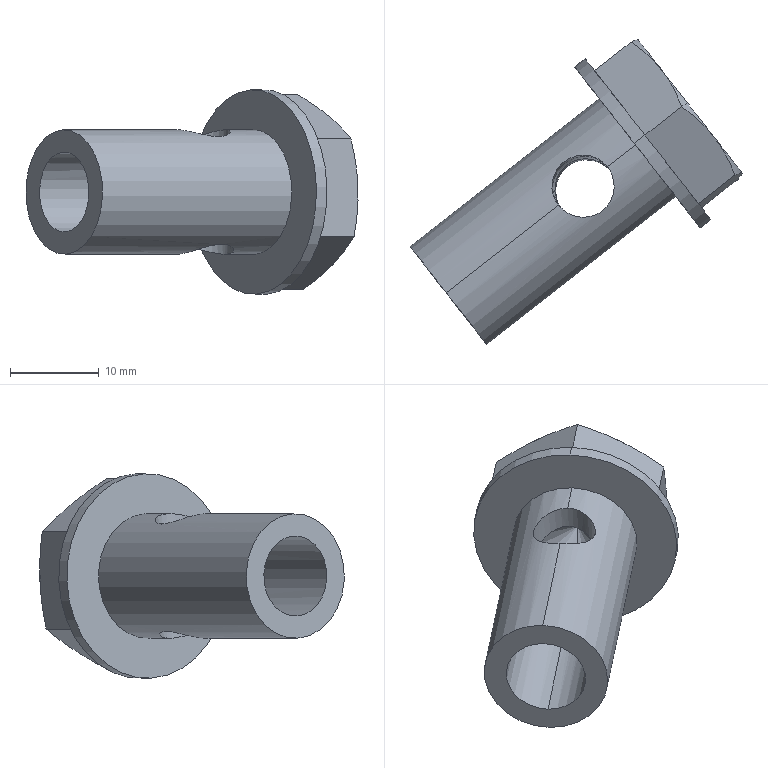Part | SolidWorks | features BaseBody 1 | 1 solid | 29 faces | box 37.348 x 34.256 x 23 mm | volume 4759 mm3 | cylinder 10 | plane 10 | cone 9 | commonest cylinder face diameters 7 x4 9 x2 14 x2 23 x2
STEP:
#1=CARTESIAN_POINT('',(4.811,97.834,81.735));
#2=VERTEX_POINT('',#1);
#3=CARTESIAN_POINT('',(5.536,96.907,58.765));
#4=VERTEX_POINT('',#3);
#5=CARTESIAN_POINT('',(5.173,97.37,70.25));
#6=DIRECTION('',(0.788,0.6157,0.));
#7=DIRECTION('',(-0.0315,0.04032,0.9987));
#8=AXIS2_PLACEMENT_3D('',#5,#6,#7);
#9=CIRCLE('',#8,11.5);
#10=EDGE_CURVE('',#2,#4,#9,.T.);
#11=ORIENTED_EDGE('',*,*,#10,.T.);
#12=CARTESIAN_POINT('',(6.718,97.83,58.765));
#13=VERTEX_POINT('',#12);
#14=CARTESIAN_POINT('',(11.446,101.524,58.765));
#15=DIRECTION('',(0.788,0.6157,0.));
#16=VECTOR('',#15,1000.);
#17=LINE('',#14,#16);
#18=EDGE_CURVE('',#4,#13,#17,.T.);
#19=ORIENTED_EDGE('',*,*,#18,.T.);
#20=CARTESIAN_POINT('',(5.993,98.757,81.735));
#21=VERTEX_POINT('',#20);
#22=CARTESIAN_POINT('',(6.355,98.294,70.25));
#23=DIRECTION('',(0.788,0.6157,0.));
#24=DIRECTION('',(0.0315,-0.04032,-0.9987));
#25=AXIS2_PLACEMENT_3D('',#22,#23,#24);
#26=CIRCLE('',#25,11.5);
#27=EDGE_CURVE('',#21,#13,#26,.T.);
#28=ORIENTED_EDGE('',*,*,#27,.F.);
#29=CARTESIAN_POINT('',(10.721,102.451,81.735));
#30=DIRECTION('',(0.788,0.6157,0.));
#31=VECTOR('',#30,1000.);
#32=LINE('',#29,#31);
#33=EDGE_CURVE('',#2,#21,#32,.T.);
#34=ORIENTED_EDGE('',*,*,#33,.F.);
#35=EDGE_LOOP('',(#11,#19,#28,#34));
#36=FACE_OUTER_BOUND('',#35,.T.);
#37=CARTESIAN_POINT('',(11.083,101.988,70.25));
#38=DIRECTION('',(0.788,0.6157,0.));
#39=DIRECTION('',(-0.0315,0.04032,0.9987));
#40=AXIS2_PLACEMENT_3D('',#37,#38,#39);
#41=CYLINDRICAL_SURFACE('',#40,11.5);
#42=ADVANCED_FACE('',(#36),#41,.T.);
#43=CARTESIAN_POINT('',(-16.323,81.03,77.241));
#44=VERTEX_POINT('',#43);
#45=CARTESIAN_POINT('',(-15.882,80.465,63.259));
#46=VERTEX_POINT('',#45);
#47=CARTESIAN_POINT('',(-16.103,80.747,70.25));
#48=DIRECTION('',(0.788,0.6157,0.));
#49=DIRECTION('',(-0.0315,0.04032,0.9987));
#50=AXIS2_PLACEMENT_3D('',#47,#48,#49);
#51=CIRCLE('',#50,7.);
#52=EDGE_CURVE('',#44,#46,#51,.T.);
#53=ORIENTED_EDGE('',*,*,#52,.T.);
#54=CARTESIAN_POINT('',(-3.274,90.316,63.259));
#55=VERTEX_POINT('',#54);
#56=CARTESIAN_POINT('',(11.304,101.705,63.259));
#57=DIRECTION('',(0.788,0.6157,0.));
#58=VECTOR('',#57,1000.);
#59=LINE('',#56,#58);
#60=EDGE_CURVE('',#46,#55,#59,.T.);
#61=ORIENTED_EDGE('',*,*,#60,.T.);
#62=CARTESIAN_POINT('',(1.606,89.754,64.375));
#63=VERTEX_POINT('',#62);
#64=CARTESIAN_POINT('',(1.606,89.754,64.375));
#65=CARTESIAN_POINT('',(1.421,89.609,64.375));
#66=CARTESIAN_POINT('',(1.22,89.482,64.359));
#67=CARTESIAN_POINT('',(0.8083,89.274,64.303));
#68=CARTESIAN_POINT('',(0.5963,89.191,64.262));
#69=CARTESIAN_POINT('',(0.1602,89.067,64.162));
#70=CARTESIAN_POINT('',(-0.0655,89.026,64.102));
#71=CARTESIAN_POINT('',(-0.5108,88.989,63.975));
#72=CARTESIAN_POINT('',(-0.7328,88.992,63.907));
#73=CARTESIAN_POINT('',(-1.177,89.042,63.77));
#74=CARTESIAN_POINT('',(-1.397,89.088,63.702));
#75=CARTESIAN_POINT('',(-1.823,89.223,63.574));
#76=CARTESIAN_POINT('',(-2.033,89.313,63.513));
#77=CARTESIAN_POINT('',(-2.431,89.534,63.408));
#78=CARTESIAN_POINT('',(-2.618,89.664,63.363));
#79=CARTESIAN_POINT('',(-2.969,89.963,63.295));
#80=CARTESIAN_POINT('',(-3.132,90.133,63.271));
#81=CARTESIAN_POINT('',(-3.274,90.316,63.259));
#82=B_SPLINE_CURVE_WITH_KNOTS('',3,(#64,#65,#66,#67,#68,#69,#70,#71,#72,#73,#74,#75,#76,#77,#78,#79,#80,#81),.UNSPECIFIED.,.F.,.F.,(4,2,2,2,2,2,2,2,4),(0.,0.0007047,0.001409,0.002114,0.002819,0.003524,0.004228,0.004933,0.005638),.UNSPECIFIED.);
#83=EDGE_CURVE('',#63,#55,#82,.T.);
#84=ORIENTED_EDGE('',*,*,#83,.F.);
#85=CARTESIAN_POINT('',(2.242,94.625,63.259));
#86=VERTEX_POINT('',#85);
#87=CARTESIAN_POINT('',(2.242,94.625,63.259));
#88=CARTESIAN_POINT('',(2.385,94.442,63.271));
#89=CARTESIAN_POINT('',(2.508,94.247,63.295));
#90=CARTESIAN_POINT('',(2.714,93.835,63.363));
#91=CARTESIAN_POINT('',(2.797,93.616,63.408));
#92=CARTESIAN_POINT('',(2.914,93.18,63.512));
#93=CARTESIAN_POINT('',(2.95,92.959,63.572));
#94=CARTESIAN_POINT('',(2.979,92.51,63.701));
#95=CARTESIAN_POINT('',(2.971,92.285,63.769));
#96=CARTESIAN_POINT('',(2.912,91.844,63.905));
#97=CARTESIAN_POINT('',(2.861,91.626,63.974));
#98=CARTESIAN_POINT('',(2.716,91.198,64.102));
#99=CARTESIAN_POINT('',(2.623,90.993,64.161));
#100=CARTESIAN_POINT('',(2.397,90.598,64.262));
#101=CARTESIAN_POINT('',(2.262,90.408,64.304));
#102=CARTESIAN_POINT('',(1.96,90.059,64.36));
#103=CARTESIAN_POINT('',(1.792,89.899,64.375));
#104=CARTESIAN_POINT('',(1.606,89.754,64.375));
#105=B_SPLINE_CURVE_WITH_KNOTS('',3,(#87,#88,#89,#90,#91,#92,#93,#94,#95,#96,#97,#98,#99,#100,#101,#102,#103,#104),.UNSPECIFIED.,.F.,.F.,(4,2,2,2,2,2,2,2,4),(0.01693,0.01764,0.01834,0.01905,0.01976,0.02046,0.02117,0.02188,0.02258),.UNSPECIFIED.);
#106=EDGE_CURVE('',#86,#63,#105,.T.);
#107=ORIENTED_EDGE('',*,*,#106,.F.);
#108=CARTESIAN_POINT('',(5.394,97.088,63.259));
#109=VERTEX_POINT('',#108);
#110=CARTESIAN_POINT('',(11.304,101.705,63.259));
#111=DIRECTION('',(0.788,0.6157,0.));
#112=VECTOR('',#111,1000.);
#113=LINE('',#110,#112);
#114=EDGE_CURVE('',#86,#109,#113,.T.);
#115=ORIENTED_EDGE('',*,*,#114,.T.);
#116=CARTESIAN_POINT('',(4.953,97.652,77.241));
#117=VERTEX_POINT('',#116);
#118=CARTESIAN_POINT('',(5.173,97.37,70.25));
#119=DIRECTION('',(0.788,0.6157,0.));
#120=DIRECTION('',(-0.0315,0.04032,0.9987));
#121=AXIS2_PLACEMENT_3D('',#118,#119,#120);
#122=CIRCLE('',#121,7.);
#123=EDGE_CURVE('',#117,#109,#122,.T.);
#124=ORIENTED_EDGE('',*,*,#123,.F.);
#125=CARTESIAN_POINT('',(1.801,95.19,77.241));
#126=VERTEX_POINT('',#125);
#127=CARTESIAN_POINT('',(10.863,102.27,77.241));
#128=DIRECTION('',(0.788,0.6157,0.));
#129=VECTOR('',#128,1000.);
#130=LINE('',#127,#129);
#131=EDGE_CURVE('',#126,#117,#130,.T.);
#132=ORIENTED_EDGE('',*,*,#131,.F.);
#133=CARTESIAN_POINT('',(1.224,90.243,76.483));
#134=VERTEX_POINT('',#133);
#135=CARTESIAN_POINT('',(1.224,90.243,76.483));
#136=CARTESIAN_POINT('',(1.41,90.388,76.483));
#137=CARTESIAN_POINT('',(1.58,90.553,76.496));
#138=CARTESIAN_POINT('',(1.879,90.906,76.543));
#139=CARTESIAN_POINT('',(2.008,91.095,76.577));
#140=CARTESIAN_POINT('',(2.228,91.495,76.659));
#141=CARTESIAN_POINT('',(2.319,91.709,76.708));
#142=CARTESIAN_POINT('',(2.455,92.141,76.81));
#143=CARTESIAN_POINT('',(2.502,92.362,76.863));
#144=CARTESIAN_POINT('',(2.554,92.815,76.967));
#145=CARTESIAN_POINT('',(2.559,93.045,77.018));
#146=CARTESIAN_POINT('',(2.524,93.499,77.107));
#147=CARTESIAN_POINT('',(2.484,93.728,77.147));
#148=CARTESIAN_POINT('',(2.361,94.175,77.209));
#149=CARTESIAN_POINT('',(2.278,94.391,77.231));
#150=CARTESIAN_POINT('',(2.07,94.808,77.253));
#151=CARTESIAN_POINT('',(1.943,95.008,77.253));
#152=CARTESIAN_POINT('',(1.801,95.19,77.241));
#153=B_SPLINE_CURVE_WITH_KNOTS('',3,(#135,#136,#137,#138,#139,#140,#141,#142,#143,#144,#145,#146,#147,#148,#149,#150,#151,#152),.UNSPECIFIED.,.F.,.F.,(4,2,2,2,2,2,2,2,4),(0.,0.0007047,0.001409,0.002114,0.002819,0.003524,0.004228,0.004933,0.005638),.UNSPECIFIED.);
#154=EDGE_CURVE('',#134,#126,#153,.T.);
#155=ORIENTED_EDGE('',*,*,#154,.F.);
#156=CARTESIAN_POINT('',(-3.715,90.88,77.241));
#157=VERTEX_POINT('',#156);
#158=CARTESIAN_POINT('',(-3.715,90.88,77.241));
#159=CARTESIAN_POINT('',(-3.572,90.697,77.253));
#160=CARTESIAN_POINT('',(-3.412,90.529,77.253));
#161=CARTESIAN_POINT('',(-3.059,90.226,77.231));
#162=CARTESIAN_POINT('',(-2.865,90.09,77.209));
#163=CARTESIAN_POINT('',(-2.464,89.864,77.148));
#164=CARTESIAN_POINT('',(-2.256,89.772,77.109));
#165=CARTESIAN_POINT('',(-1.82,89.626,77.018));
#166=CARTESIAN_POINT('',(-1.596,89.575,76.968));
#167=CARTESIAN_POINT('',(-1.147,89.516,76.864));
#168=CARTESIAN_POINT('',(-0.9184,89.507,76.81));
#169=CARTESIAN_POINT('',(-0.4615,89.535,76.708));
#170=CARTESIAN_POINT('',(-0.2367,89.571,76.66));
#171=CARTESIAN_POINT('',(0.2071,89.688,76.577));
#172=CARTESIAN_POINT('',(0.4272,89.77,76.543));
#173=CARTESIAN_POINT('',(0.8417,89.975,76.496));
#174=CARTESIAN_POINT('',(1.038,90.097,76.483));
#175=CARTESIAN_POINT('',(1.224,90.243,76.483));
#176=B_SPLINE_CURVE_WITH_KNOTS('',3,(#158,#159,#160,#161,#162,#163,#164,#165,#166,#167,#168,#169,#170,#171,#172,#173,#174,#175),.UNSPECIFIED.,.F.,.F.,(4,2,2,2,2,2,2,2,4),(0.01693,0.01764,0.01834,0.01905,0.01976,0.02046,0.02117,0.02188,0.02258),.UNSPECIFIED.);
#177=EDGE_CURVE('',#157,#134,#176,.T.);
#178=ORIENTED_EDGE('',*,*,#177,.F.);
#179=CARTESIAN_POINT('',(10.863,102.27,77.241));
#180=DIRECTION('',(0.788,0.6157,0.));
#181=VECTOR('',#180,1000.);
#182=LINE('',#179,#181);
#183=EDGE_CURVE('',#44,#157,#182,.T.);
#184=ORIENTED_EDGE('',*,*,#183,.F.);
#185=EDGE_LOOP('',(#53,#61,#84,#107,#115,#124,#132,#155,#178,#184));
#186=FACE_OUTER_BOUND('',#185,.T.);
#187=CARTESIAN_POINT('',(11.083,101.988,70.25));
#188=DIRECTION('',(0.788,0.6157,0.));
#189=DIRECTION('',(-0.0315,0.04032,0.9987));
#190=AXIS2_PLACEMENT_3D('',#187,#188,#189);
#191=CYLINDRICAL_SURFACE('',#190,7.);
#192=ADVANCED_FACE('',(#186),#191,.T.);
#193=CARTESIAN_POINT('',(-15.961,80.566,65.756));
#194=VERTEX_POINT('',#193);
#195=CARTESIAN_POINT('',(-16.245,80.929,74.744));
#196=VERTEX_POINT('',#195);
#197=CARTESIAN_POINT('',(-16.103,80.747,70.25));
#198=DIRECTION('',(0.788,0.6157,0.));
#199=DIRECTION('',(-0.0315,0.04032,0.9987));
#200=AXIS2_PLACEMENT_3D('',#197,#198,#199);
#201=CIRCLE('',#200,4.5);
#202=EDGE_CURVE('',#194,#196,#201,.T.);
#203=ORIENTED_EDGE('',*,*,#202,.F.);
#204=CARTESIAN_POINT('',(-3.353,90.416,65.756));
#205=VERTEX_POINT('',#204);
#206=CARTESIAN_POINT('',(11.225,101.806,65.756));
#207=DIRECTION('',(0.788,0.6157,0.));
#208=VECTOR('',#207,1000.);
#209=LINE('',#206,#208);
#210=EDGE_CURVE('',#194,#205,#209,.T.);
#211=ORIENTED_EDGE('',*,*,#210,.T.);
#212=CARTESIAN_POINT('',(-2.8,95.393,67.246));
#213=VERTEX_POINT('',#212);
#214=CARTESIAN_POINT('',(-2.8,95.393,67.246));
#215=CARTESIAN_POINT('',(-2.992,95.243,67.246));
#216=CARTESIAN_POINT('',(-3.163,95.076,67.216));
#217=CARTESIAN_POINT('',(-3.466,94.709,67.107));
#218=CARTESIAN_POINT('',(-3.592,94.517,67.032));
#219=CARTESIAN_POINT('',(-3.803,94.118,66.861));
#220=CARTESIAN_POINT('',(-3.888,93.909,66.765));
#221=CARTESIAN_POINT('',(-4.017,93.487,66.573));
#222=CARTESIAN_POINT('',(-4.062,93.273,66.475));
#223=CARTESIAN_POINT('',(-4.112,92.832,66.287));
#224=CARTESIAN_POINT('',(-4.118,92.604,66.196));
#225=CARTESIAN_POINT('',(-4.086,92.152,66.035));
#226=CARTESIAN_POINT('',(-4.049,91.925,65.963));
#227=CARTESIAN_POINT('',(-3.927,91.469,65.846));
#228=CARTESIAN_POINT('',(-3.844,91.245,65.802));
#229=CARTESIAN_POINT('',(-3.632,90.815,65.751));
#230=CARTESIAN_POINT('',(-3.501,90.606,65.744));
#231=CARTESIAN_POINT('',(-3.353,90.416,65.756));
#232=B_SPLINE_CURVE_WITH_KNOTS('',3,(#214,#215,#216,#217,#218,#219,#220,#221,#222,#223,#224,#225,#226,#227,#228,#229,#230,#231),.UNSPECIFIED.,.F.,.F.,(4,2,2,2,2,2,2,2,4),(0.0115,0.01222,0.01294,0.01366,0.01438,0.0151,0.01582,0.01654,0.01726),.UNSPECIFIED.);
#233=EDGE_CURVE('',#213,#205,#232,.T.);
#234=ORIENTED_EDGE('',*,*,#233,.F.);
#235=CARTESIAN_POINT('',(2.163,94.726,65.756));
#236=VERTEX_POINT('',#235);
#237=CARTESIAN_POINT('',(2.163,94.726,65.756));
#238=CARTESIAN_POINT('',(2.015,94.915,65.744));
#239=CARTESIAN_POINT('',(1.848,95.09,65.751));
#240=CARTESIAN_POINT('',(1.479,95.402,65.802));
#241=CARTESIAN_POINT('',(1.283,95.536,65.846));
#242=CARTESIAN_POINT('',(0.8722,95.764,65.962));
#243=CARTESIAN_POINT('',(0.658,95.856,66.034));
#244=CARTESIAN_POINT('',(0.2264,95.997,66.196));
#245=CARTESIAN_POINT('',(0.005111,96.047,66.287));
#246=CARTESIAN_POINT('',(-0.4358,96.105,66.475));
#247=CARTESIAN_POINT('',(-0.6555,96.114,66.573));
#248=CARTESIAN_POINT('',(-1.097,96.091,66.766));
#249=CARTESIAN_POINT('',(-1.32,96.058,66.862));
#250=CARTESIAN_POINT('',(-1.757,95.95,67.032));
#251=CARTESIAN_POINT('',(-1.976,95.873,67.107));
#252=CARTESIAN_POINT('',(-2.403,95.669,67.215));
#253=CARTESIAN_POINT('',(-2.608,95.543,67.246));
#254=CARTESIAN_POINT('',(-2.8,95.393,67.246));
#255=B_SPLINE_CURVE_WITH_KNOTS('',3,(#237,#238,#239,#240,#241,#242,#243,#244,#245,#246,#247,#248,#249,#250,#251,#252,#253,#254),.UNSPECIFIED.,.F.,.F.,(4,2,2,2,2,2,2,2,4),(0.005755,0.006473,0.007192,0.00791,0.008628,0.009347,0.01007,0.01078,0.0115),.UNSPECIFIED.);
#256=EDGE_CURVE('',#236,#213,#255,.T.);
#257=ORIENTED_EDGE('',*,*,#256,.F.);
#258=CARTESIAN_POINT('',(3.739,95.957,65.756));
#259=VERTEX_POINT('',#258);
#260=CARTESIAN_POINT('',(11.225,101.806,65.756));
#261=DIRECTION('',(0.788,0.6157,0.));
#262=VECTOR('',#261,1000.);
#263=LINE('',#260,#262);
#264=EDGE_CURVE('',#236,#259,#263,.T.);
#265=ORIENTED_EDGE('',*,*,#264,.T.);
#266=CARTESIAN_POINT('',(3.456,96.32,74.744));
#267=VERTEX_POINT('',#266);
#268=CARTESIAN_POINT('',(3.597,96.139,70.25));
#269=DIRECTION('',(0.788,0.6157,0.));
#270=DIRECTION('',(-0.0315,0.04032,0.9987));
#271=AXIS2_PLACEMENT_3D('',#268,#269,#270);
#272=CIRCLE('',#271,4.5);
#273=EDGE_CURVE('',#259,#267,#272,.T.);
#274=ORIENTED_EDGE('',*,*,#273,.T.);
#275=CARTESIAN_POINT('',(1.88,95.089,74.744));
#276=VERTEX_POINT('',#275);
#277=CARTESIAN_POINT('',(10.942,102.169,74.744));
#278=DIRECTION('',(0.788,0.6157,0.));
#279=VECTOR('',#278,1000.);
#280=LINE('',#277,#279);
#281=EDGE_CURVE('',#276,#267,#280,.T.);
#282=ORIENTED_EDGE('',*,*,#281,.F.);
#283=CARTESIAN_POINT('',(-2.978,95.621,72.896));
#284=VERTEX_POINT('',#283);
#285=CARTESIAN_POINT('',(-2.978,95.621,72.896));
#286=CARTESIAN_POINT('',(-2.786,95.771,72.896));
#287=CARTESIAN_POINT('',(-2.584,95.899,72.929));
#288=CARTESIAN_POINT('',(-2.162,96.114,73.047));
#289=CARTESIAN_POINT('',(-1.95,96.196,73.13));
#290=CARTESIAN_POINT('',(-1.523,96.319,73.318));
#291=CARTESIAN_POINT('',(-1.306,96.36,73.425));
#292=CARTESIAN_POINT('',(-0.8789,96.399,73.642));
#293=CARTESIAN_POINT('',(-0.6663,96.399,73.754));
#294=CARTESIAN_POINT('',(-0.239,96.358,73.973));
#295=CARTESIAN_POINT('',(-0.02332,96.316,74.082));
#296=CARTESIAN_POINT('',(0.3965,96.19,74.281));
#297=CARTESIAN_POINT('',(0.6024,96.105,74.373));
#298=CARTESIAN_POINT('',(1.007,95.888,74.533));
#299=CARTESIAN_POINT('',(1.2,95.758,74.6));
#300=CARTESIAN_POINT('',(1.562,95.454,74.699));
#301=CARTESIAN_POINT('',(1.732,95.278,74.732));
#302=CARTESIAN_POINT('',(1.88,95.089,74.744));
#303=B_SPLINE_CURVE_WITH_KNOTS('',3,(#285,#286,#287,#288,#289,#290,#291,#292,#293,#294,#295,#296,#297,#298,#299,#300,#301,#302),.UNSPECIFIED.,.F.,.F.,(4,2,2,2,2,2,2,2,4),(0.0115,0.01222,0.01294,0.01366,0.01438,0.0151,0.01582,0.01654,0.01726),.UNSPECIFIED.);
#304=EDGE_CURVE('',#284,#276,#303,.T.);
#305=ORIENTED_EDGE('',*,*,#304,.F.);
#306=CARTESIAN_POINT('',(-3.637,90.779,74.744));
#307=VERTEX_POINT('',#306);
#308=CARTESIAN_POINT('',(-3.637,90.779,74.744));
#309=CARTESIAN_POINT('',(-3.784,90.969,74.732));
#310=CARTESIAN_POINT('',(-3.912,91.172,74.7));
#311=CARTESIAN_POINT('',(-4.121,91.599,74.6));
#312=CARTESIAN_POINT('',(-4.2,91.817,74.534));
#313=CARTESIAN_POINT('',(-4.313,92.26,74.375));
#314=CARTESIAN_POINT('',(-4.345,92.483,74.282));
#315=CARTESIAN_POINT('',(-4.366,92.921,74.082));
#316=CARTESIAN_POINT('',(-4.355,93.14,73.974));
#317=CARTESIAN_POINT('',(-4.292,93.566,73.754));
#318=CARTESIAN_POINT('',(-4.241,93.773,73.643));
#319=CARTESIAN_POINT('',(-4.098,94.179,73.425));
#320=CARTESIAN_POINT('',(-4.007,94.379,73.318));
#321=CARTESIAN_POINT('',(-3.784,94.763,73.13));
#322=CARTESIAN_POINT('',(-3.652,94.95,73.047));
#323=CARTESIAN_POINT('',(-3.344,95.305,72.929));
#324=CARTESIAN_POINT('',(-3.17,95.471,72.896));
#325=CARTESIAN_POINT('',(-2.978,95.621,72.896));
#326=B_SPLINE_CURVE_WITH_KNOTS('',3,(#308,#309,#310,#311,#312,#313,#314,#315,#316,#317,#318,#319,#320,#321,#322,#323,#324,#325),.UNSPECIFIED.,.F.,.F.,(4,2,2,2,2,2,2,2,4),(0.005755,0.006473,0.007192,0.00791,0.008628,0.009347,0.01007,0.01078,0.0115),.UNSPECIFIED.);
#327=EDGE_CURVE('',#307,#284,#326,.T.);
#328=ORIENTED_EDGE('',*,*,#327,.F.);
#329=CARTESIAN_POINT('',(10.942,102.169,74.744));
#330=DIRECTION('',(0.788,0.6157,0.));
#331=VECTOR('',#330,1000.);
#332=LINE('',#329,#331);
#333=EDGE_CURVE('',#196,#307,#332,.T.);
#334=ORIENTED_EDGE('',*,*,#333,.F.);
#335=EDGE_LOOP('',(#203,#211,#234,#257,#265,#274,#282,#305,#328,#334));
#336=FACE_OUTER_BOUND('',#335,.T.);
#337=CARTESIAN_POINT('',(11.083,101.988,70.25));
#338=DIRECTION('',(0.788,0.6157,0.));
#339=DIRECTION('',(-0.0315,0.04032,0.9987));
#340=AXIS2_PLACEMENT_3D('',#337,#338,#339);
#341=CYLINDRICAL_SURFACE('',#340,4.5);
#342=ADVANCED_FACE('',(#336),#341,.F.);
#343=CARTESIAN_POINT('',(7.124,98.894,70.25));
#344=VERTEX_POINT('',#343);
#345=CARTESIAN_POINT('',(3.739,95.957,65.756));
#346=DIRECTION('',(-0.5333,-0.4627,-0.7082));
#347=VECTOR('',#346,1000.);
#348=LINE('',#345,#347);
#349=EDGE_CURVE('',#344,#259,#348,.T.);
#350=ORIENTED_EDGE('',*,*,#349,.F.);
#351=CARTESIAN_POINT('',(3.456,96.32,74.744));
#352=DIRECTION('',(-0.578,-0.4055,0.7082));
#353=VECTOR('',#352,1000.);
#354=LINE('',#351,#353);
#355=EDGE_CURVE('',#344,#267,#354,.T.);
#356=ORIENTED_EDGE('',*,*,#355,.T.);
#357=ORIENTED_EDGE('',*,*,#273,.F.);
#358=EDGE_LOOP('',(#350,#356,#357));
#359=FACE_OUTER_BOUND('',#358,.T.);
#360=CARTESIAN_POINT('',(3.597,96.139,70.25));
#361=DIRECTION('',(-0.788,-0.6157,0.));
#362=DIRECTION('',(0.0315,-0.04032,-0.9987));
#363=AXIS2_PLACEMENT_3D('',#360,#361,#362);
#364=CONICAL_SURFACE('',#363,4.5,0.7882);
#365=ADVANCED_FACE('',(#359),#364,.F.);
#366=CARTESIAN_POINT('',(10.784,102.371,79.738));
#367=VERTEX_POINT('',#366);
#368=CARTESIAN_POINT('',(13.745,98.581,78.71));
#369=VERTEX_POINT('',#368);
#370=CARTESIAN_POINT('',(11.083,101.988,70.25));
#371=DIRECTION('',(0.788,0.6157,0.));
#372=DIRECTION('',(-0.0315,0.04032,0.9987));
#373=AXIS2_PLACEMENT_3D('',#370,#371,#372);
#374=CIRCLE('',#373,9.5);
#375=EDGE_CURVE('',#367,#369,#374,.T.);
#376=ORIENTED_EDGE('',*,*,#375,.F.);
#377=CARTESIAN_POINT('',(10.122,101.949,81.205));
#378=VERTEX_POINT('',#377);
#379=CARTESIAN_POINT('',(10.784,102.371,79.738));
#380=DIRECTION('',(-0.3978,-0.2534,0.8818));
#381=VECTOR('',#380,1000.);
#382=LINE('',#379,#381);
#383=EDGE_CURVE('',#367,#378,#382,.T.);
#384=ORIENTED_EDGE('',*,*,#383,.T.);
#385=CARTESIAN_POINT('',(13.745,98.581,78.71));
#386=CARTESIAN_POINT('',(13.234,99.236,79.134));
#387=CARTESIAN_POINT('',(12.669,99.837,79.554));
#388=CARTESIAN_POINT('',(11.454,100.952,80.385));
#389=CARTESIAN_POINT('',(10.803,101.465,80.796));
#390=CARTESIAN_POINT('',(10.122,101.949,81.205));
#391=B_SPLINE_CURVE_WITH_KNOTS('',3,(#385,#386,#387,#388,#389,#390),.UNSPECIFIED.,.F.,.F.,(4,2,4),(0.,0.00277,0.00554),.UNSPECIFIED.);
#392=EDGE_CURVE('',#369,#378,#391,.T.);
#393=ORIENTED_EDGE('',*,*,#392,.F.);
#394=EDGE_LOOP('',(#376,#384,#393));
#395=FACE_OUTER_BOUND('',#394,.T.);
#396=CARTESIAN_POINT('',(11.083,101.988,70.25));
#397=DIRECTION('',(-0.788,-0.6157,0.));
#398=DIRECTION('',(-0.0315,0.04032,0.9987));
#399=AXIS2_PLACEMENT_3D('',#396,#397,#398);
#400=CONICAL_SURFACE('',#399,9.5,1.082);
#401=ADVANCED_FACE('',(#395),#400,.T.);
#402=CARTESIAN_POINT('',(1.504,89.884,67.604));
#403=VERTEX_POINT('',#402);
#404=CARTESIAN_POINT('',(1.504,89.884,67.604));
#405=CARTESIAN_POINT('',(1.698,90.035,67.604));
#406=CARTESIAN_POINT('',(1.869,90.199,67.571));
#407=CARTESIAN_POINT('',(2.099,90.464,67.484));
#408=CARTESIAN_POINT('',(2.172,90.556,67.448));
#409=CARTESIAN_POINT('',(2.305,90.743,67.368));
#410=CARTESIAN_POINT('',(2.366,90.837,67.324));
#411=CARTESIAN_POINT('',(2.532,91.125,67.183));
#412=CARTESIAN_POINT('',(2.623,91.322,67.078));
#413=CARTESIAN_POINT('',(2.767,91.732,66.858));
#414=CARTESIAN_POINT('',(2.818,91.939,66.746));
#415=CARTESIAN_POINT('',(2.881,92.363,66.527));
#416=CARTESIAN_POINT('',(2.893,92.583,66.418));
#417=CARTESIAN_POINT('',(2.872,93.022,66.219));
#418=CARTESIAN_POINT('',(2.84,93.242,66.127));
#419=CARTESIAN_POINT('',(2.728,93.684,65.967));
#420=CARTESIAN_POINT('',(2.648,93.906,65.9));
#421=CARTESIAN_POINT('',(2.441,94.329,65.801));
#422=CARTESIAN_POINT('',(2.311,94.536,65.768));
#423=CARTESIAN_POINT('',(2.163,94.726,65.756));
#424=B_SPLINE_CURVE_WITH_KNOTS('',3,(#404,#405,#406,#407,#408,#409,#410,#411,#412,#413,#414,#415,#416,#417,#418,#419,#420,#421,#422,#423),.UNSPECIFIED.,.F.,.F.,(4,2,2,2,2,2,2,2,2,4),(0.,0.0007194,0.001079,0.001439,0.002158,0.002878,0.003597,0.004316,0.005036,0.005755),.UNSPECIFIED.);
#425=EDGE_CURVE('',#403,#236,#424,.T.);
#426=ORIENTED_EDGE('',*,*,#425,.T.);
#427=ORIENTED_EDGE('',*,*,#256,.T.);
#428=CARTESIAN_POINT('',(-2.698,95.263,64.017));
#429=VERTEX_POINT('',#428);
#430=CARTESIAN_POINT('',(-3.204,95.91,80.058));
#431=DIRECTION('',(0.0315,-0.04032,-0.9987));
#432=VECTOR('',#431,1000.);
#433=LINE('',#430,#432);
#434=EDGE_CURVE('',#213,#429,#433,.T.);
#435=ORIENTED_EDGE('',*,*,#434,.T.);
#436=CARTESIAN_POINT('',(-2.698,95.263,64.017));
#437=CARTESIAN_POINT('',(-2.515,95.406,64.017));
#438=CARTESIAN_POINT('',(-2.319,95.529,64.005));
#439=CARTESIAN_POINT('',(-1.901,95.736,63.958));
#440=CARTESIAN_POINT('',(-1.683,95.817,63.923));
#441=CARTESIAN_POINT('',(-1.243,95.933,63.841));
#442=CARTESIAN_POINT('',(-1.017,95.969,63.793));
#443=CARTESIAN_POINT('',(-0.5598,95.998,63.691));
#444=CARTESIAN_POINT('',(-0.3335,95.99,63.637));
#445=CARTESIAN_POINT('',(0.1159,95.932,63.534));
#446=CARTESIAN_POINT('',(0.3412,95.88,63.483));
#447=CARTESIAN_POINT('',(0.7757,95.736,63.393));
#448=CARTESIAN_POINT('',(0.9855,95.644,63.353));
#449=CARTESIAN_POINT('',(1.39,95.416,63.291));
#450=CARTESIAN_POINT('',(1.582,95.282,63.269));
#451=CARTESIAN_POINT('',(1.935,94.98,63.247));
#452=CARTESIAN_POINT('',(2.098,94.809,63.247));
#453=CARTESIAN_POINT('',(2.242,94.625,63.259));
#454=B_SPLINE_CURVE_WITH_KNOTS('',3,(#436,#437,#438,#439,#440,#441,#442,#443,#444,#445,#446,#447,#448,#449,#450,#451,#452,#453),.UNSPECIFIED.,.F.,.F.,(4,2,2,2,2,2,2,2,4),(0.01128,0.01199,0.01269,0.0134,0.01411,0.01481,0.01552,0.01622,0.01693),.UNSPECIFIED.);
#455=EDGE_CURVE('',#429,#86,#454,.T.);
#456=ORIENTED_EDGE('',*,*,#455,.T.);
#457=ORIENTED_EDGE('',*,*,#106,.T.);
#458=CARTESIAN_POINT('',(1.1,90.402,80.416));
#459=DIRECTION('',(0.0315,-0.04032,-0.9987));
#460=VECTOR('',#459,1000.);
#461=LINE('',#458,#460);
#462=EDGE_CURVE('',#403,#63,#461,.T.);
#463=ORIENTED_EDGE('',*,*,#462,.F.);
#464=EDGE_LOOP('',(#426,#427,#435,#456,#457,#463));
#465=FACE_OUTER_BOUND('',#464,.T.);
#466=CARTESIAN_POINT('',(-1.052,93.156,80.237));
#467=DIRECTION('',(0.0315,-0.04032,-0.9987));
#468=DIRECTION('',(0.6149,-0.787,0.05117));
#469=AXIS2_PLACEMENT_3D('',#466,#467,#468);
#470=CYLINDRICAL_SURFACE('',#469,3.5);
#471=ADVANCED_FACE('',(#465),#470,.F.);
#472=ORIENTED_EDGE('',*,*,#154,.T.);
#473=CARTESIAN_POINT('',(-3.08,95.752,76.125));
#474=VERTEX_POINT('',#473);
#475=CARTESIAN_POINT('',(1.801,95.19,77.241));
#476=CARTESIAN_POINT('',(1.658,95.372,77.229));
#477=CARTESIAN_POINT('',(1.497,95.541,77.205));
#478=CARTESIAN_POINT('',(1.144,95.842,77.136));
#479=CARTESIAN_POINT('',(0.957,95.972,77.092));
#480=CARTESIAN_POINT('',(0.5625,96.191,76.988));
#481=CARTESIAN_POINT('',(0.3527,96.281,76.927));
#482=CARTESIAN_POINT('',(-0.07493,96.417,76.799));
#483=CARTESIAN_POINT('',(-0.2921,96.463,76.731));
#484=CARTESIAN_POINT('',(-0.7344,96.513,76.595));
#485=CARTESIAN_POINT('',(-0.9609,96.516,76.526));
#486=CARTESIAN_POINT('',(-1.407,96.479,76.398));
#487=CARTESIAN_POINT('',(-1.629,96.439,76.339));
#488=CARTESIAN_POINT('',(-2.071,96.314,76.237));
#489=CARTESIAN_POINT('',(-2.284,96.231,76.196));
#490=CARTESIAN_POINT('',(-2.697,96.022,76.14));
#491=CARTESIAN_POINT('',(-2.897,95.894,76.125));
#492=CARTESIAN_POINT('',(-3.08,95.752,76.125));
#493=B_SPLINE_CURVE_WITH_KNOTS('',3,(#475,#476,#477,#478,#479,#480,#481,#482,#483,#484,#485,#486,#487,#488,#489,#490,#491,#492),.UNSPECIFIED.,.F.,.F.,(4,2,2,2,2,2,2,2,4),(0.005638,0.006343,0.007049,0.007754,0.00846,0.009165,0.009871,0.01058,0.01128),.UNSPECIFIED.);
#494=EDGE_CURVE('',#126,#474,#493,.T.);
#495=ORIENTED_EDGE('',*,*,#494,.T.);
#496=CARTESIAN_POINT('',(-3.204,95.91,80.058));
#497=DIRECTION('',(0.0315,-0.04032,-0.9987));
#498=VECTOR('',#497,1000.);
#499=LINE('',#496,#498);
#500=EDGE_CURVE('',#474,#284,#499,.T.);
#501=ORIENTED_EDGE('',*,*,#500,.T.);
#502=ORIENTED_EDGE('',*,*,#304,.T.);
#503=CARTESIAN_POINT('',(1.326,90.112,73.254));
#504=VERTEX_POINT('',#503);
#505=CARTESIAN_POINT('',(1.88,95.089,74.744));
#506=CARTESIAN_POINT('',(2.027,94.9,74.756));
#507=CARTESIAN_POINT('',(2.157,94.693,74.749));
#508=CARTESIAN_POINT('',(2.37,94.261,74.698));
#509=CARTESIAN_POINT('',(2.453,94.039,74.654));
#510=CARTESIAN_POINT('',(2.575,93.584,74.538));
#511=CARTESIAN_POINT('',(2.612,93.355,74.466));
#512=CARTESIAN_POINT('',(2.644,92.901,74.304));
#513=CARTESIAN_POINT('',(2.639,92.674,74.213));
#514=CARTESIAN_POINT('',(2.589,92.233,74.024));
#515=CARTESIAN_POINT('',(2.544,92.017,73.927));
#516=CARTESIAN_POINT('',(2.414,91.593,73.733));
#517=CARTESIAN_POINT('',(2.329,91.385,73.638));
#518=CARTESIAN_POINT('',(2.171,91.087,73.51));
#519=CARTESIAN_POINT('',(2.112,90.989,73.47));
#520=CARTESIAN_POINT('',(1.985,90.797,73.398));
#521=CARTESIAN_POINT('',(1.914,90.702,73.365));
#522=CARTESIAN_POINT('',(1.689,90.43,73.284));
#523=CARTESIAN_POINT('',(1.519,90.263,73.254));
#524=CARTESIAN_POINT('',(1.326,90.112,73.254));
#525=B_SPLINE_CURVE_WITH_KNOTS('',3,(#505,#506,#507,#508,#509,#510,#511,#512,#513,#514,#515,#516,#517,#518,#519,#520,#521,#522,#523,#524),.UNSPECIFIED.,.F.,.F.,(4,2,2,2,2,2,2,2,2,4),(0.01726,0.01797,0.01869,0.01941,0.02013,0.02085,0.02157,0.02193,0.02228,0.023),.UNSPECIFIED.);
#526=EDGE_CURVE('',#276,#504,#525,.T.);
#527=ORIENTED_EDGE('',*,*,#526,.T.);
#528=CARTESIAN_POINT('',(1.1,90.402,80.416));
#529=DIRECTION('',(0.0315,-0.04032,-0.9987));
#530=VECTOR('',#529,1000.);
#531=LINE('',#528,#530);
#532=EDGE_CURVE('',#134,#504,#531,.T.);
#533=ORIENTED_EDGE('',*,*,#532,.F.);
#534=EDGE_LOOP('',(#472,#495,#501,#502,#527,#533));
#535=FACE_OUTER_BOUND('',#534,.T.);
#536=CARTESIAN_POINT('',(-1.052,93.156,80.237));
#537=DIRECTION('',(0.0315,-0.04032,-0.9987));
#538=DIRECTION('',(0.6149,-0.787,0.05117));
#539=AXIS2_PLACEMENT_3D('',#536,#537,#538);
#540=CYLINDRICAL_SURFACE('',#539,3.5);
#541=ADVANCED_FACE('',(#535),#540,.F.);
#542=ORIENTED_EDGE('',*,*,#500,.F.);
#543=CARTESIAN_POINT('',(-3.08,95.752,76.125));
#544=CARTESIAN_POINT('',(-3.262,95.609,76.125));
#545=CARTESIAN_POINT('',(-3.43,95.45,76.14));
#546=CARTESIAN_POINT('',(-3.735,95.098,76.196));
#547=CARTESIAN_POINT('',(-3.869,94.909,76.237));
#548=CARTESIAN_POINT('',(-4.094,94.517,76.337));
#549=CARTESIAN_POINT('',(-4.187,94.312,76.396));
#550=CARTESIAN_POINT('',(-4.333,93.884,76.525));
#551=CARTESIAN_POINT('',(-4.384,93.668,76.593));
#552=CARTESIAN_POINT('',(-4.444,93.227,76.729));
#553=CARTESIAN_POINT('',(-4.452,93.001,76.798));
#554=CARTESIAN_POINT('',(-4.424,92.553,76.926));
#555=CARTESIAN_POINT('',(-4.389,92.332,76.986));
#556=CARTESIAN_POINT('',(-4.271,91.891,77.092));
#557=CARTESIAN_POINT('',(-4.189,91.674,77.137));
#558=CARTESIAN_POINT('',(-3.984,91.263,77.205));
#559=CARTESIAN_POINT('',(-3.859,91.064,77.229));
#560=CARTESIAN_POINT('',(-3.715,90.88,77.241));
#561=B_SPLINE_CURVE_WITH_KNOTS('',3,(#543,#544,#545,#546,#547,#548,#549,#550,#551,#552,#553,#554,#555,#556,#557,#558,#559,#560),.UNSPECIFIED.,.F.,.F.,(4,2,2,2,2,2,2,2,4),(0.01128,0.01199,0.01269,0.0134,0.01411,0.01481,0.01552,0.01622,0.01693),.UNSPECIFIED.);
#562=EDGE_CURVE('',#474,#157,#561,.T.);
#563=ORIENTED_EDGE('',*,*,#562,.T.);
#564=ORIENTED_EDGE('',*,*,#177,.T.);
#565=ORIENTED_EDGE('',*,*,#532,.T.);
#566=CARTESIAN_POINT('',(1.326,90.112,73.254));
#567=CARTESIAN_POINT('',(1.133,89.961,73.254));
#568=CARTESIAN_POINT('',(0.9301,89.837,73.285));
#569=CARTESIAN_POINT('',(0.6122,89.685,73.365));
#570=CARTESIAN_POINT('',(0.5031,89.639,73.397));
#571=CARTESIAN_POINT('',(0.2851,89.562,73.47));
#572=CARTESIAN_POINT('',(0.1762,89.529,73.51));
#573=CARTESIAN_POINT('',(-0.1515,89.448,73.638));
#574=CARTESIAN_POINT('',(-0.3714,89.415,73.732));
#575=CARTESIAN_POINT('',(-0.8164,89.392,73.927));
#576=CARTESIAN_POINT('',(-1.037,89.4,74.025));
#577=CARTESIAN_POINT('',(-1.477,89.458,74.213));
#578=CARTESIAN_POINT('',(-1.698,89.508,74.304));
#579=CARTESIAN_POINT('',(-2.131,89.649,74.466));
#580=CARTESIAN_POINT('',(-2.342,89.74,74.537));
#581=CARTESIAN_POINT('',(-2.753,89.967,74.653));
#582=CARTESIAN_POINT('',(-2.952,90.103,74.698));
#583=CARTESIAN_POINT('',(-3.317,90.412,74.749));
#584=CARTESIAN_POINT('',(-3.488,90.59,74.756));
#585=CARTESIAN_POINT('',(-3.637,90.779,74.744));
#586=B_SPLINE_CURVE_WITH_KNOTS('',3,(#566,#567,#568,#569,#570,#571,#572,#573,#574,#575,#576,#577,#578,#579,#580,#581,#582,#583,#584,#585),.UNSPECIFIED.,.F.,.F.,(4,2,2,2,2,2,2,2,2,4),(0.,0.0007194,0.001079,0.001439,0.002158,0.002878,0.003597,0.004316,0.005036,0.005755),.UNSPECIFIED.);
#587=EDGE_CURVE('',#504,#307,#586,.T.);
#588=ORIENTED_EDGE('',*,*,#587,.T.);
#589=ORIENTED_EDGE('',*,*,#327,.T.);
#590=EDGE_LOOP('',(#542,#563,#564,#565,#588,#589));
#591=FACE_OUTER_BOUND('',#590,.T.);
#592=CARTESIAN_POINT('',(-1.052,93.156,80.237));
#593=DIRECTION('',(0.0315,-0.04032,-0.9987));
#594=DIRECTION('',(0.6149,-0.787,0.05117));
#595=AXIS2_PLACEMENT_3D('',#592,#593,#594);
#596=CYLINDRICAL_SURFACE('',#595,3.5);
#597=ADVANCED_FACE('',(#591),#596,.F.);
#598=ORIENTED_EDGE('',*,*,#434,.F.);
#599=ORIENTED_EDGE('',*,*,#233,.T.);
#600=CARTESIAN_POINT('',(-3.353,90.416,65.756));
#601=CARTESIAN_POINT('',(-3.205,90.227,65.768));
#602=CARTESIAN_POINT('',(-3.037,90.053,65.8));
#603=CARTESIAN_POINT('',(-2.674,89.748,65.9));
#604=CARTESIAN_POINT('',(-2.482,89.618,65.966));
#605=CARTESIAN_POINT('',(-2.079,89.401,66.126));
#606=CARTESIAN_POINT('',(-1.871,89.316,66.219));
#607=CARTESIAN_POINT('',(-1.45,89.19,66.418));
#608=CARTESIAN_POINT('',(-1.235,89.148,66.527));
#609=CARTESIAN_POINT('',(-0.807,89.107,66.746));
#610=CARTESIAN_POINT('',(-0.5937,89.106,66.858));
#611=CARTESIAN_POINT('',(-0.1634,89.146,67.077));
#612=CARTESIAN_POINT('',(0.05193,89.187,67.183));
#613=CARTESIAN_POINT('',(0.3712,89.279,67.324));
#614=CARTESIAN_POINT('',(0.4774,89.315,67.368));
#615=CARTESIAN_POINT('',(0.6901,89.399,67.448));
#616=CARTESIAN_POINT('',(0.7972,89.447,67.483));
#617=CARTESIAN_POINT('',(1.11,89.606,67.571));
#618=CARTESIAN_POINT('',(1.312,89.734,67.604));
#619=CARTESIAN_POINT('',(1.504,89.884,67.604));
#620=B_SPLINE_CURVE_WITH_KNOTS('',3,(#600,#601,#602,#603,#604,#605,#606,#607,#608,#609,#610,#611,#612,#613,#614,#615,#616,#617,#618,#619),.UNSPECIFIED.,.F.,.F.,(4,2,2,2,2,2,2,2,2,4),(0.01726,0.01797,0.01869,0.01941,0.02013,0.02085,0.02157,0.02193,0.02228,0.023),.UNSPECIFIED.);
#621=EDGE_CURVE('',#205,#403,#620,.T.);
#622=ORIENTED_EDGE('',*,*,#621,.T.);
#623=ORIENTED_EDGE('',*,*,#462,.T.);
#624=ORIENTED_EDGE('',*,*,#83,.T.);
#625=CARTESIAN_POINT('',(-3.274,90.316,63.259));
#626=CARTESIAN_POINT('',(-3.417,90.498,63.247));
#627=CARTESIAN_POINT('',(-3.542,90.696,63.247));
#628=CARTESIAN_POINT('',(-3.752,91.115,63.269));
#629=CARTESIAN_POINT('',(-3.834,91.331,63.291));
#630=CARTESIAN_POINT('',(-3.957,91.773,63.352));
#631=CARTESIAN_POINT('',(-3.997,92.003,63.392));
#632=CARTESIAN_POINT('',(-4.032,92.459,63.482));
#633=CARTESIAN_POINT('',(-4.028,92.686,63.532));
#634=CARTESIAN_POINT('',(-3.977,93.137,63.636));
#635=CARTESIAN_POINT('',(-3.929,93.363,63.69));
#636=CARTESIAN_POINT('',(-3.793,93.796,63.792));
#637=CARTESIAN_POINT('',(-3.704,94.006,63.84));
#638=CARTESIAN_POINT('',(-3.481,94.412,63.923));
#639=CARTESIAN_POINT('',(-3.351,94.602,63.957));
#640=CARTESIAN_POINT('',(-3.052,94.955,64.004));
#641=CARTESIAN_POINT('',(-2.88,95.12,64.017));
#642=CARTESIAN_POINT('',(-2.698,95.263,64.017));
#643=B_SPLINE_CURVE_WITH_KNOTS('',3,(#625,#626,#627,#628,#629,#630,#631,#632,#633,#634,#635,#636,#637,#638,#639,#640,#641,#642),.UNSPECIFIED.,.F.,.F.,(4,2,2,2,2,2,2,2,4),(0.005638,0.006343,0.007049,0.007754,0.00846,0.009165,0.009871,0.01058,0.01128),.UNSPECIFIED.);
#644=EDGE_CURVE('',#55,#429,#643,.T.);
#645=ORIENTED_EDGE('',*,*,#644,.T.);
#646=EDGE_LOOP('',(#598,#599,#622,#623,#624,#645));
#647=FACE_OUTER_BOUND('',#646,.T.);
#648=CARTESIAN_POINT('',(-1.052,93.156,80.237));
#649=DIRECTION('',(0.0315,-0.04032,-0.9987));
#650=DIRECTION('',(0.6149,-0.787,0.05117));
#651=AXIS2_PLACEMENT_3D('',#648,#649,#650);
#652=CYLINDRICAL_SURFACE('',#651,3.5);
#653=ADVANCED_FACE('',(#647),#652,.F.);
#654=CARTESIAN_POINT('',(7.904,106.058,78.223));
#655=VERTEX_POINT('',#654);
#656=CARTESIAN_POINT('',(11.083,101.988,70.25));
#657=DIRECTION('',(0.788,0.6157,0.));
#658=DIRECTION('',(-0.0315,0.04032,0.9987));
#659=AXIS2_PLACEMENT_3D('',#656,#657,#658);
#660=CIRCLE('',#659,9.5);
#661=EDGE_CURVE('',#655,#367,#660,.T.);
#662=ORIENTED_EDGE('',*,*,#661,.T.);
#663=ORIENTED_EDGE('',*,*,#375,.T.);
#664=CARTESIAN_POINT('',(16.925,94.511,70.736));
#665=VERTEX_POINT('',#664);
#666=CARTESIAN_POINT('',(11.083,101.988,70.25));
#667=DIRECTION('',(0.788,0.6157,0.));
#668=DIRECTION('',(-0.0315,0.04032,0.9987));
#669=AXIS2_PLACEMENT_3D('',#666,#667,#668);
#670=CIRCLE('',#669,9.5);
#671=EDGE_CURVE('',#369,#665,#670,.T.);
#672=ORIENTED_EDGE('',*,*,#671,.T.);
#673=CARTESIAN_POINT('',(14.263,97.918,62.277));
#674=VERTEX_POINT('',#673);
#675=CARTESIAN_POINT('',(11.083,101.988,70.25));
#676=DIRECTION('',(0.788,0.6157,0.));
#677=DIRECTION('',(-0.0315,0.04032,0.9987));
#678=AXIS2_PLACEMENT_3D('',#675,#676,#677);
#679=CIRCLE('',#678,9.5);
#680=EDGE_CURVE('',#665,#674,#679,.T.);
#681=ORIENTED_EDGE('',*,*,#680,.T.);
#682=CARTESIAN_POINT('',(8.422,105.394,61.79));
#683=VERTEX_POINT('',#682);
#684=CARTESIAN_POINT('',(11.083,101.988,70.25));
#685=DIRECTION('',(0.788,0.6157,0.));
#686=DIRECTION('',(-0.0315,0.04032,0.9987));
#687=AXIS2_PLACEMENT_3D('',#684,#685,#686);
#688=CIRCLE('',#687,9.5);
#689=EDGE_CURVE('',#674,#683,#688,.T.);
#690=ORIENTED_EDGE('',*,*,#689,.T.);
#691=CARTESIAN_POINT('',(5.242,109.464,69.764));
#692=VERTEX_POINT('',#691);
#693=CARTESIAN_POINT('',(11.083,101.988,70.25));
#694=DIRECTION('',(0.788,0.6157,0.));
#695=DIRECTION('',(-0.0315,0.04032,0.9987));
#696=AXIS2_PLACEMENT_3D('',#693,#694,#695);
#697=CIRCLE('',#696,9.5);
#698=EDGE_CURVE('',#683,#692,#697,.T.);
#699=ORIENTED_EDGE('',*,*,#698,.T.);
#700=CARTESIAN_POINT('',(11.083,101.988,70.25));
#701=DIRECTION('',(0.788,0.6157,0.));
#702=DIRECTION('',(-0.0315,0.04032,0.9987));
#703=AXIS2_PLACEMENT_3D('',#700,#701,#702);
#704=CIRCLE('',#703,9.5);
#705=EDGE_CURVE('',#692,#655,#704,.T.);
#706=ORIENTED_EDGE('',*,*,#705,.T.);
#707=EDGE_LOOP('',(#662,#663,#672,#681,#690,#699,#706));
#708=FACE_OUTER_BOUND('',#707,.T.);
#709=CARTESIAN_POINT('',(11.083,101.988,70.25));
#710=DIRECTION('',(0.788,0.6157,0.));
#711=DIRECTION('',(0.,0.,-1.));
#712=AXIS2_PLACEMENT_3D('',#709,#710,#711);
#713=PLANE('',#712);
#714=ADVANCED_FACE('',(#708),#713,.T.);
#715=ORIENTED_EDGE('',*,*,#671,.F.);
#716=CARTESIAN_POINT('',(16.136,94.251,76.214));
#717=VERTEX_POINT('',#716);
#718=CARTESIAN_POINT('',(16.136,94.251,76.214));
#719=CARTESIAN_POINT('',(15.832,95.029,76.623));
#720=CARTESIAN_POINT('',(15.491,95.785,77.034));
#721=CARTESIAN_POINT('',(14.703,97.234,77.866));
#722=CARTESIAN_POINT('',(14.256,97.927,78.285));
#723=CARTESIAN_POINT('',(13.745,98.581,78.71));
#724=B_SPLINE_CURVE_WITH_KNOTS('',3,(#718,#719,#720,#721,#722,#723),.UNSPECIFIED.,.F.,.F.,(4,2,4),(0.,0.00277,0.00554),.UNSPECIFIED.);
#725=EDGE_CURVE('',#717,#369,#724,.T.);
#726=ORIENTED_EDGE('',*,*,#725,.F.);
#727=CARTESIAN_POINT('',(16.925,94.511,70.736));
#728=CARTESIAN_POINT('',(16.895,94.549,71.668));
#729=CARTESIAN_POINT('',(16.808,94.54,72.588));
#730=CARTESIAN_POINT('',(16.536,94.447,74.413));
#731=CARTESIAN_POINT('',(16.353,94.362,75.316));
#732=CARTESIAN_POINT('',(16.136,94.251,76.214));
#733=B_SPLINE_CURVE_WITH_KNOTS('',3,(#727,#728,#729,#730,#731,#732),.UNSPECIFIED.,.F.,.F.,(4,2,4),(0.,0.00277,0.00554),.UNSPECIFIED.);
#734=EDGE_CURVE('',#665,#717,#733,.T.);
#735=ORIENTED_EDGE('',*,*,#734,.F.);
#736=EDGE_LOOP('',(#715,#726,#735));
#737=FACE_OUTER_BOUND('',#736,.T.);
#738=CARTESIAN_POINT('',(11.083,101.988,70.25));
#739=DIRECTION('',(-0.788,-0.6157,0.));
#740=DIRECTION('',(-0.0315,0.04032,0.9987));
#741=AXIS2_PLACEMENT_3D('',#738,#739,#740);
#742=CONICAL_SURFACE('',#741,9.5,1.082);
#743=ADVANCED_FACE('',(#737),#742,.T.);
#744=ORIENTED_EDGE('',*,*,#680,.F.);
#745=CARTESIAN_POINT('',(16.482,93.809,65.258));
#746=VERTEX_POINT('',#745);
#747=CARTESIAN_POINT('',(16.482,93.809,65.258));
#748=CARTESIAN_POINT('',(16.642,93.992,66.156));
#749=CARTESIAN_POINT('',(16.768,94.15,67.059));
#750=CARTESIAN_POINT('',(16.925,94.391,68.884));
#751=CARTESIAN_POINT('',(16.954,94.474,69.805));
#752=CARTESIAN_POINT('',(16.925,94.511,70.736));
#753=B_SPLINE_CURVE_WITH_KNOTS('',3,(#747,#748,#749,#750,#751,#752),.UNSPECIFIED.,.F.,.F.,(4,2,4),(0.,0.00277,0.00554),.UNSPECIFIED.);
#754=EDGE_CURVE('',#746,#665,#753,.T.);
#755=ORIENTED_EDGE('',*,*,#754,.F.);
#756=CARTESIAN_POINT('',(14.263,97.918,62.277));
#757=CARTESIAN_POINT('',(14.745,97.301,62.784));
#758=CARTESIAN_POINT('',(15.163,96.645,63.285));
#759=CARTESIAN_POINT('',(15.893,95.27,64.278));
#760=CARTESIAN_POINT('',(16.205,94.551,64.77));
#761=CARTESIAN_POINT('',(16.482,93.809,65.258));
#762=B_SPLINE_CURVE_WITH_KNOTS('',3,(#756,#757,#758,#759,#760,#761),.UNSPECIFIED.,.F.,.F.,(4,2,4),(0.,0.00277,0.00554),.UNSPECIFIED.);
#763=EDGE_CURVE('',#674,#746,#762,.T.);
#764=ORIENTED_EDGE('',*,*,#763,.F.);
#765=EDGE_LOOP('',(#744,#755,#764));
#766=FACE_OUTER_BOUND('',#765,.T.);
#767=CARTESIAN_POINT('',(11.083,101.988,70.25));
#768=DIRECTION('',(-0.788,-0.6157,0.));
#769=DIRECTION('',(-0.0315,0.04032,0.9987));
#770=AXIS2_PLACEMENT_3D('',#767,#768,#769);
#771=CONICAL_SURFACE('',#770,9.5,1.082);
#772=ADVANCED_FACE('',(#766),#771,.T.);
#773=ORIENTED_EDGE('',*,*,#689,.F.);
#774=CARTESIAN_POINT('',(10.813,101.064,59.295));
#775=VERTEX_POINT('',#774);
#776=CARTESIAN_POINT('',(10.813,101.064,59.295));
#777=CARTESIAN_POINT('',(11.466,100.617,59.783));
#778=CARTESIAN_POINT('',(12.088,100.14,60.275));
#779=CARTESIAN_POINT('',(13.246,99.099,61.268));
#780=CARTESIAN_POINT('',(13.781,98.535,61.77));
#781=CARTESIAN_POINT('',(14.263,97.918,62.277));
#782=B_SPLINE_CURVE_WITH_KNOTS('',3,(#776,#777,#778,#779,#780,#781),.UNSPECIFIED.,.F.,.F.,(4,2,4),(0.,0.00277,0.00554),.UNSPECIFIED.);
#783=EDGE_CURVE('',#775,#674,#782,.T.);
#784=ORIENTED_EDGE('',*,*,#783,.F.);
#785=CARTESIAN_POINT('',(8.422,105.394,61.79));
#786=CARTESIAN_POINT('',(8.933,104.74,61.366));
#787=CARTESIAN_POINT('',(9.38,104.047,60.946));
#788=CARTESIAN_POINT('',(10.168,102.598,60.115));
#789=CARTESIAN_POINT('',(10.509,101.842,59.704));
#790=CARTESIAN_POINT('',(10.813,101.064,59.295));
#791=B_SPLINE_CURVE_WITH_KNOTS('',3,(#785,#786,#787,#788,#789,#790),.UNSPECIFIED.,.F.,.F.,(4,2,4),(0.,0.00277,0.00554),.UNSPECIFIED.);
#792=EDGE_CURVE('',#683,#775,#791,.T.);
#793=ORIENTED_EDGE('',*,*,#792,.F.);
#794=EDGE_LOOP('',(#773,#784,#793));
#795=FACE_OUTER_BOUND('',#794,.T.);
#796=CARTESIAN_POINT('',(11.083,101.988,70.25));
#797=DIRECTION('',(-0.788,-0.6157,0.));
#798=DIRECTION('',(-0.0315,0.04032,0.9987));
#799=AXIS2_PLACEMENT_3D('',#796,#797,#798);
#800=CONICAL_SURFACE('',#799,9.5,1.082);
#801=ADVANCED_FACE('',(#795),#800,.T.);
#802=ORIENTED_EDGE('',*,*,#698,.F.);
#803=CARTESIAN_POINT('',(4.799,108.762,64.286));
#804=VERTEX_POINT('',#803);
#805=CARTESIAN_POINT('',(4.799,108.762,64.286));
#806=CARTESIAN_POINT('',(5.48,108.278,63.877));
#807=CARTESIAN_POINT('',(6.131,107.764,63.466));
#808=CARTESIAN_POINT('',(7.347,106.65,62.634));
#809=CARTESIAN_POINT('',(7.911,106.049,62.215));
#810=CARTESIAN_POINT('',(8.422,105.394,61.79));
#811=B_SPLINE_CURVE_WITH_KNOTS('',3,(#805,#806,#807,#808,#809,#810),.UNSPECIFIED.,.F.,.F.,(4,2,4),(0.,0.00277,0.00554),.UNSPECIFIED.);
#812=EDGE_CURVE('',#804,#683,#811,.T.);
#813=ORIENTED_EDGE('',*,*,#812,.F.);
#814=CARTESIAN_POINT('',(5.242,109.464,69.764));
#815=CARTESIAN_POINT('',(5.272,109.426,68.832));
#816=CARTESIAN_POINT('',(5.242,109.343,67.912));
#817=CARTESIAN_POINT('',(5.086,109.103,66.087));
#818=CARTESIAN_POINT('',(4.959,108.945,65.184));
#819=CARTESIAN_POINT('',(4.799,108.762,64.286));
#820=B_SPLINE_CURVE_WITH_KNOTS('',3,(#814,#815,#816,#817,#818,#819),.UNSPECIFIED.,.F.,.F.,(4,2,4),(0.,0.00277,0.00554),.UNSPECIFIED.);
#821=EDGE_CURVE('',#692,#804,#820,.T.);
#822=ORIENTED_EDGE('',*,*,#821,.F.);
#823=EDGE_LOOP('',(#802,#813,#822));
#824=FACE_OUTER_BOUND('',#823,.T.);
#825=CARTESIAN_POINT('',(11.083,101.988,70.25));
#826=DIRECTION('',(-0.788,-0.6157,0.));
#827=DIRECTION('',(-0.0315,0.04032,0.9987));
#828=AXIS2_PLACEMENT_3D('',#825,#826,#827);
#829=CONICAL_SURFACE('',#828,9.5,1.082);
#830=ADVANCED_FACE('',(#824),#829,.T.);
#831=ORIENTED_EDGE('',*,*,#705,.F.);
#832=CARTESIAN_POINT('',(4.454,109.204,75.242));
#833=VERTEX_POINT('',#832);
#834=CARTESIAN_POINT('',(4.454,109.204,75.242));
#835=CARTESIAN_POINT('',(4.67,109.315,74.344));
#836=CARTESIAN_POINT('',(4.854,109.399,73.441));
#837=CARTESIAN_POINT('',(5.125,109.493,71.616));
#838=CARTESIAN_POINT('',(5.213,109.502,70.695));
#839=CARTESIAN_POINT('',(5.242,109.464,69.764));
#840=B_SPLINE_CURVE_WITH_KNOTS('',3,(#834,#835,#836,#837,#838,#839),.UNSPECIFIED.,.F.,.F.,(4,2,4),(0.,0.00277,0.00554),.UNSPECIFIED.);
#841=EDGE_CURVE('',#833,#692,#840,.T.);
#842=ORIENTED_EDGE('',*,*,#841,.F.);
#843=CARTESIAN_POINT('',(7.904,106.058,78.223));
#844=CARTESIAN_POINT('',(7.422,106.674,77.716));
#845=CARTESIAN_POINT('',(6.887,107.239,77.215));
#846=CARTESIAN_POINT('',(5.729,108.279,76.222));
#847=CARTESIAN_POINT('',(5.106,108.757,75.73));
#848=CARTESIAN_POINT('',(4.454,109.204,75.242));
#849=B_SPLINE_CURVE_WITH_KNOTS('',3,(#843,#844,#845,#846,#847,#848),.UNSPECIFIED.,.F.,.F.,(4,2,4),(0.,0.00277,0.00554),.UNSPECIFIED.);
#850=EDGE_CURVE('',#655,#833,#849,.T.);
#851=ORIENTED_EDGE('',*,*,#850,.F.);
#852=EDGE_LOOP('',(#831,#842,#851));
#853=FACE_OUTER_BOUND('',#852,.T.);
#854=CARTESIAN_POINT('',(11.083,101.988,70.25));
#855=DIRECTION('',(-0.788,-0.6157,0.));
#856=DIRECTION('',(-0.0315,0.04032,0.9987));
#857=AXIS2_PLACEMENT_3D('',#854,#855,#856);
#858=CONICAL_SURFACE('',#857,9.5,1.082);
#859=ADVANCED_FACE('',(#853),#858,.T.);
#860=ORIENTED_EDGE('',*,*,#383,.F.);
#861=ORIENTED_EDGE('',*,*,#661,.F.);
#862=CARTESIAN_POINT('',(10.122,101.949,81.205));
#863=CARTESIAN_POINT('',(9.846,102.69,80.717));
#864=CARTESIAN_POINT('',(9.533,103.41,80.225));
#865=CARTESIAN_POINT('',(8.804,104.785,79.232));
#866=CARTESIAN_POINT('',(8.386,105.441,78.73));
#867=CARTESIAN_POINT('',(7.904,106.058,78.223));
#868=B_SPLINE_CURVE_WITH_KNOTS('',3,(#862,#863,#864,#865,#866,#867),.UNSPECIFIED.,.F.,.F.,(4,2,4),(0.,0.00277,0.00554),.UNSPECIFIED.);
#869=EDGE_CURVE('',#378,#655,#868,.T.);
#870=ORIENTED_EDGE('',*,*,#869,.F.);
#871=EDGE_LOOP('',(#860,#861,#870));
#872=FACE_OUTER_BOUND('',#871,.T.);
#873=CARTESIAN_POINT('',(11.083,101.988,70.25));
#874=DIRECTION('',(-0.788,-0.6157,0.));
#875=DIRECTION('',(-0.0315,0.04032,0.9987));
#876=AXIS2_PLACEMENT_3D('',#873,#874,#875);
#877=CONICAL_SURFACE('',#876,9.5,1.082);
#878=ADVANCED_FACE('',(#872),#877,.T.);
#879=CARTESIAN_POINT('',(0.687,105.549,64.286));
#880=VERTEX_POINT('',#879);
#881=CARTESIAN_POINT('',(0.3415,105.991,75.242));
#882=VERTEX_POINT('',#881);
#883=CARTESIAN_POINT('',(0.687,105.549,64.286));
#884=DIRECTION('',(-0.0315,0.04032,0.9987));
#885=VECTOR('',#884,1000.);
#886=LINE('',#883,#885);
#887=EDGE_CURVE('',#880,#882,#886,.T.);
#888=ORIENTED_EDGE('',*,*,#887,.F.);
#889=CARTESIAN_POINT('',(6.701,97.851,59.295));
#890=VERTEX_POINT('',#889);
#891=CARTESIAN_POINT('',(6.701,97.851,59.295));
#892=DIRECTION('',(-0.5482,0.7017,0.455));
#893=VECTOR('',#892,1000.);
#894=LINE('',#891,#893);
#895=EDGE_CURVE('',#890,#880,#894,.T.);
#896=ORIENTED_EDGE('',*,*,#895,.F.);
#897=CARTESIAN_POINT('',(12.369,90.596,65.258));
#898=VERTEX_POINT('',#897);
#899=CARTESIAN_POINT('',(12.369,90.596,65.258));
#900=DIRECTION('',(-0.5167,0.6614,-0.5437));
#901=VECTOR('',#900,1000.);
#902=LINE('',#899,#901);
#903=EDGE_CURVE('',#898,#890,#902,.T.);
#904=ORIENTED_EDGE('',*,*,#903,.F.);
#905=CARTESIAN_POINT('',(12.024,91.039,76.214));
#906=VERTEX_POINT('',#905);
#907=CARTESIAN_POINT('',(12.024,91.039,76.214));
#908=DIRECTION('',(0.0315,-0.04032,-0.9987));
#909=VECTOR('',#908,1000.);
#910=LINE('',#907,#909);
#911=EDGE_CURVE('',#906,#898,#910,.T.);
#912=ORIENTED_EDGE('',*,*,#911,.F.);
#913=CARTESIAN_POINT('',(6.01,98.736,81.205));
#914=VERTEX_POINT('',#913);
#915=CARTESIAN_POINT('',(6.01,98.736,81.205));
#916=DIRECTION('',(0.5482,-0.7017,-0.455));
#917=VECTOR('',#916,1000.);
#918=LINE('',#915,#917);
#919=EDGE_CURVE('',#914,#906,#918,.T.);
#920=ORIENTED_EDGE('',*,*,#919,.F.);
#921=CARTESIAN_POINT('',(0.3415,105.991,75.242));
#922=DIRECTION('',(0.5167,-0.6614,0.5437));
#923=VECTOR('',#922,1000.);
#924=LINE('',#921,#923);
#925=EDGE_CURVE('',#882,#914,#924,.T.);
#926=ORIENTED_EDGE('',*,*,#925,.F.);
#927=EDGE_LOOP('',(#888,#896,#904,#912,#920,#926));
#928=FACE_BOUND('',#927,.T.);
#929=ORIENTED_EDGE('',*,*,#27,.T.);
#930=CARTESIAN_POINT('',(6.355,98.294,70.25));
#931=DIRECTION('',(0.788,0.6157,0.));
#932=DIRECTION('',(0.0315,-0.04032,-0.9987));
#933=AXIS2_PLACEMENT_3D('',#930,#931,#932);
#934=CIRCLE('',#933,11.5);
#935=EDGE_CURVE('',#13,#21,#934,.T.);
#936=ORIENTED_EDGE('',*,*,#935,.T.);
#937=EDGE_LOOP('',(#929,#936));
#938=FACE_OUTER_BOUND('',#937,.T.);
#939=CARTESIAN_POINT('',(16.267,85.607,71.075));
#940=DIRECTION('',(-0.788,-0.6157,0.));
#941=DIRECTION('',(-0.6157,0.788,0.));
#942=AXIS2_PLACEMENT_3D('',#939,#940,#941);
#943=PLANE('',#942);
#944=ADVANCED_FACE('',(#928,#938),#943,.F.);
#945=ORIENTED_EDGE('',*,*,#355,.F.);
#946=ORIENTED_EDGE('',*,*,#349,.T.);
#947=CARTESIAN_POINT('',(3.597,96.139,70.25));
#948=DIRECTION('',(0.788,0.6157,0.));
#949=DIRECTION('',(-0.0315,0.04032,0.9987));
#950=AXIS2_PLACEMENT_3D('',#947,#948,#949);
#951=CIRCLE('',#950,4.5);
#952=EDGE_CURVE('',#267,#259,#951,.T.);
#953=ORIENTED_EDGE('',*,*,#952,.F.);
#954=EDGE_LOOP('',(#945,#946,#953));
#955=FACE_OUTER_BOUND('',#954,.T.);
#956=CARTESIAN_POINT('',(3.597,96.139,70.25));
#957=DIRECTION('',(-0.788,-0.6157,0.));
#958=DIRECTION('',(0.0315,-0.04032,-0.9987));
#959=AXIS2_PLACEMENT_3D('',#956,#957,#958);
#960=CONICAL_SURFACE('',#959,4.5,0.7882);
#961=ADVANCED_FACE('',(#955),#960,.F.);
#962=ORIENTED_EDGE('',*,*,#210,.F.);
#963=CARTESIAN_POINT('',(-16.103,80.747,70.25));
#964=DIRECTION('',(0.788,0.6157,0.));
#965=DIRECTION('',(-0.0315,0.04032,0.9987));
#966=AXIS2_PLACEMENT_3D('',#963,#964,#965);
#967=CIRCLE('',#966,4.5);
#968=EDGE_CURVE('',#196,#194,#967,.T.);
#969=ORIENTED_EDGE('',*,*,#968,.F.);
#970=ORIENTED_EDGE('',*,*,#333,.T.);
#971=ORIENTED_EDGE('',*,*,#587,.F.);
#972=ORIENTED_EDGE('',*,*,#526,.F.);
#973=ORIENTED_EDGE('',*,*,#281,.T.);
#974=ORIENTED_EDGE('',*,*,#952,.T.);
#975=ORIENTED_EDGE('',*,*,#264,.F.);
#976=ORIENTED_EDGE('',*,*,#425,.F.);
#977=ORIENTED_EDGE('',*,*,#621,.F.);
#978=EDGE_LOOP('',(#962,#969,#970,#971,#972,#973,#974,#975,#976,#977));
#979=FACE_OUTER_BOUND('',#978,.T.);
#980=CARTESIAN_POINT('',(11.083,101.988,70.25));
#981=DIRECTION('',(0.788,0.6157,0.));
#982=DIRECTION('',(-0.0315,0.04032,0.9987));
#983=AXIS2_PLACEMENT_3D('',#980,#981,#982);
#984=CYLINDRICAL_SURFACE('',#983,4.5);
#985=ADVANCED_FACE('',(#979),#984,.F.);
#986=ORIENTED_EDGE('',*,*,#52,.F.);
#987=CARTESIAN_POINT('',(-16.103,80.747,70.25));
#988=DIRECTION('',(0.788,0.6157,0.));
#989=DIRECTION('',(-0.0315,0.04032,0.9987));
#990=AXIS2_PLACEMENT_3D('',#987,#988,#989);
#991=CIRCLE('',#990,7.);
#992=EDGE_CURVE('',#46,#44,#991,.T.);
#993=ORIENTED_EDGE('',*,*,#992,.F.);
#994=EDGE_LOOP('',(#986,#993));
#995=FACE_OUTER_BOUND('',#994,.T.);
#996=ORIENTED_EDGE('',*,*,#968,.T.);
#997=ORIENTED_EDGE('',*,*,#202,.T.);
#998=EDGE_LOOP('',(#996,#997));
#999=FACE_BOUND('',#998,.T.);
#1000=CARTESIAN_POINT('',(-11.799,75.238,70.608));
#1001=DIRECTION('',(-0.788,-0.6157,0.));
#1002=DIRECTION('',(-0.6157,0.788,0.));
#1003=AXIS2_PLACEMENT_3D('',#1000,#1001,#1002);
#1004=PLANE('',#1003);
#1005=ADVANCED_FACE('',(#995,#999),#1004,.T.);
#1006=ORIENTED_EDGE('',*,*,#60,.F.);
#1007=ORIENTED_EDGE('',*,*,#992,.T.);
#1008=ORIENTED_EDGE('',*,*,#183,.T.);
#1009=ORIENTED_EDGE('',*,*,#562,.F.);
#1010=ORIENTED_EDGE('',*,*,#494,.F.);
#1011=ORIENTED_EDGE('',*,*,#131,.T.);
#1012=CARTESIAN_POINT('',(5.173,97.37,70.25));
#1013=DIRECTION('',(0.788,0.6157,0.));
#1014=DIRECTION('',(-0.0315,0.04032,0.9987));
#1015=AXIS2_PLACEMENT_3D('',#1012,#1013,#1014);
#1016=CIRCLE('',#1015,7.);
#1017=EDGE_CURVE('',#109,#117,#1016,.T.);
#1018=ORIENTED_EDGE('',*,*,#1017,.F.);
#1019=ORIENTED_EDGE('',*,*,#114,.F.);
#1020=ORIENTED_EDGE('',*,*,#455,.F.);
#1021=ORIENTED_EDGE('',*,*,#644,.F.);
#1022=EDGE_LOOP('',(#1006,#1007,#1008,#1009,#1010,#1011,#1018,#1019,#1020,#1021));
#1023=FACE_OUTER_BOUND('',#1022,.T.);
#1024=CARTESIAN_POINT('',(11.083,101.988,70.25));
#1025=DIRECTION('',(0.788,0.6157,0.));
#1026=DIRECTION('',(-0.0315,0.04032,0.9987));
#1027=AXIS2_PLACEMENT_3D('',#1024,#1025,#1026);
#1028=CYLINDRICAL_SURFACE('',#1027,7.);
#1029=ADVANCED_FACE('',(#1023),#1028,.T.);
#1030=ORIENTED_EDGE('',*,*,#10,.F.);
#1031=CARTESIAN_POINT('',(5.173,97.37,70.25));
#1032=DIRECTION('',(0.788,0.6157,0.));
#1033=DIRECTION('',(-0.0315,0.04032,0.9987));
#1034=AXIS2_PLACEMENT_3D('',#1031,#1032,#1033);
#1035=CIRCLE('',#1034,11.5);
#1036=EDGE_CURVE('',#4,#2,#1035,.T.);
#1037=ORIENTED_EDGE('',*,*,#1036,.F.);
#1038=EDGE_LOOP('',(#1030,#1037));
#1039=FACE_OUTER_BOUND('',#1038,.T.);
#1040=ORIENTED_EDGE('',*,*,#123,.T.);
#1041=ORIENTED_EDGE('',*,*,#1017,.T.);
#1042=EDGE_LOOP('',(#1040,#1041));
#1043=FACE_BOUND('',#1042,.T.);
#1044=CARTESIAN_POINT('',(12.244,88.32,70.838));
#1045=DIRECTION('',(-0.788,-0.6157,0.));
#1046=DIRECTION('',(-0.6157,0.788,0.));
#1047=AXIS2_PLACEMENT_3D('',#1044,#1045,#1046);
#1048=PLANE('',#1047);
#1049=ADVANCED_FACE('',(#1039,#1043),#1048,.T.);
#1050=ORIENTED_EDGE('',*,*,#18,.F.);
#1051=ORIENTED_EDGE('',*,*,#1036,.T.);
#1052=ORIENTED_EDGE('',*,*,#33,.T.);
#1053=ORIENTED_EDGE('',*,*,#935,.F.);
#1054=EDGE_LOOP('',(#1050,#1051,#1052,#1053));
#1055=FACE_OUTER_BOUND('',#1054,.T.);
#1056=CARTESIAN_POINT('',(11.083,101.988,70.25));
#1057=DIRECTION('',(0.788,0.6157,0.));
#1058=DIRECTION('',(-0.0315,0.04032,0.9987));
#1059=AXIS2_PLACEMENT_3D('',#1056,#1057,#1058);
#1060=CYLINDRICAL_SURFACE('',#1059,11.5);
#1061=ADVANCED_FACE('',(#1055),#1060,.T.);
#1062=CARTESIAN_POINT('',(-166.283,-48.27,76.214));
#1063=DIRECTION('',(0.788,0.6157,0.));
#1064=VECTOR('',#1063,1000.);
#1065=LINE('',#1062,#1064);
#1066=EDGE_CURVE('',#906,#717,#1065,.T.);
#1067=ORIENTED_EDGE('',*,*,#1066,.T.);
#1068=ORIENTED_EDGE('',*,*,#725,.T.);
#1069=ORIENTED_EDGE('',*,*,#392,.T.);
#1070=CARTESIAN_POINT('',(-172.297,-40.572,81.205));
#1071=DIRECTION('',(0.788,0.6157,0.));
#1072=VECTOR('',#1071,1000.);
#1073=LINE('',#1070,#1072);
#1074=EDGE_CURVE('',#914,#378,#1073,.T.);
#1075=ORIENTED_EDGE('',*,*,#1074,.F.);
#1076=ORIENTED_EDGE('',*,*,#919,.T.);
#1077=EDGE_LOOP('',(#1067,#1068,#1069,#1075,#1076));
#1078=FACE_OUTER_BOUND('',#1077,.T.);
#1079=CARTESIAN_POINT('',(-172.297,-40.572,81.205));
#1080=DIRECTION('',(0.2801,-0.3586,0.8905));
#1081=DIRECTION('',(-0.788,-0.6157,0.));
#1082=AXIS2_PLACEMENT_3D('',#1079,#1080,#1081);
#1083=PLANE('',#1082);
#1084=ADVANCED_FACE('',(#1078),#1083,.T.);
#1085=CARTESIAN_POINT('',(-165.937,-48.712,65.258));
#1086=DIRECTION('',(0.788,0.6157,0.));
#1087=VECTOR('',#1086,1000.);
#1088=LINE('',#1085,#1087);
#1089=EDGE_CURVE('',#898,#746,#1088,.T.);
#1090=ORIENTED_EDGE('',*,*,#1089,.T.);
#1091=ORIENTED_EDGE('',*,*,#754,.T.);
#1092=ORIENTED_EDGE('',*,*,#734,.T.);
#1093=ORIENTED_EDGE('',*,*,#1066,.F.);
#1094=ORIENTED_EDGE('',*,*,#911,.T.);
#1095=EDGE_LOOP('',(#1090,#1091,#1092,#1093,#1094));
#1096=FACE_OUTER_BOUND('',#1095,.T.);
#1097=CARTESIAN_POINT('',(-166.283,-48.27,76.214));
#1098=DIRECTION('',(0.6149,-0.787,0.05117));
#1099=DIRECTION('',(0.,-0.06488,-0.9979));
#1100=AXIS2_PLACEMENT_3D('',#1097,#1098,#1099);
#1101=PLANE('',#1100);
#1102=ADVANCED_FACE('',(#1096),#1101,.T.);
#1103=CARTESIAN_POINT('',(-171.605,-41.457,59.295));
#1104=DIRECTION('',(0.788,0.6157,0.));
#1105=VECTOR('',#1104,1000.);
#1106=LINE('',#1103,#1105);
#1107=EDGE_CURVE('',#890,#775,#1106,.T.);
#1108=ORIENTED_EDGE('',*,*,#1107,.T.);
#1109=ORIENTED_EDGE('',*,*,#783,.T.);
#1110=ORIENTED_EDGE('',*,*,#763,.T.);
#1111=ORIENTED_EDGE('',*,*,#1089,.F.);
#1112=ORIENTED_EDGE('',*,*,#903,.T.);
#1113=EDGE_LOOP('',(#1108,#1109,#1110,#1111,#1112));
#1114=FACE_OUTER_BOUND('',#1113,.T.);
#1115=CARTESIAN_POINT('',(-165.937,-48.712,65.258));
#1116=DIRECTION('',(0.3347,-0.4284,-0.8393));
#1117=DIRECTION('',(0.,-0.8907,0.4546));
#1118=AXIS2_PLACEMENT_3D('',#1115,#1116,#1117);
#1119=PLANE('',#1118);
#1120=ADVANCED_FACE('',(#1114),#1119,.T.);
#1121=CARTESIAN_POINT('',(-177.619,-33.759,64.286));
#1122=DIRECTION('',(0.788,0.6157,0.));
#1123=VECTOR('',#1122,1000.);
#1124=LINE('',#1121,#1123);
#1125=EDGE_CURVE('',#880,#804,#1124,.T.);
#1126=ORIENTED_EDGE('',*,*,#1125,.T.);
#1127=ORIENTED_EDGE('',*,*,#812,.T.);
#1128=ORIENTED_EDGE('',*,*,#792,.T.);
#1129=ORIENTED_EDGE('',*,*,#1107,.F.);
#1130=ORIENTED_EDGE('',*,*,#895,.T.);
#1131=EDGE_LOOP('',(#1126,#1127,#1128,#1129,#1130));
#1132=FACE_OUTER_BOUND('',#1131,.T.);
#1133=CARTESIAN_POINT('',(-171.605,-41.457,59.295));
#1134=DIRECTION('',(-0.2801,0.3586,-0.8905));
#1135=DIRECTION('',(-0.9539,0.,0.3001));
#1136=AXIS2_PLACEMENT_3D('',#1133,#1134,#1135);
#1137=PLANE('',#1136);
#1138=ADVANCED_FACE('',(#1132),#1137,.T.);
#1139=CARTESIAN_POINT('',(-177.965,-33.317,75.242));
#1140=DIRECTION('',(0.788,0.6157,0.));
#1141=VECTOR('',#1140,1000.);
#1142=LINE('',#1139,#1141);
#1143=EDGE_CURVE('',#882,#833,#1142,.T.);
#1144=ORIENTED_EDGE('',*,*,#1143,.T.);
#1145=ORIENTED_EDGE('',*,*,#841,.T.);
#1146=ORIENTED_EDGE('',*,*,#821,.T.);
#1147=ORIENTED_EDGE('',*,*,#1125,.F.);
#1148=ORIENTED_EDGE('',*,*,#887,.T.);
#1149=EDGE_LOOP('',(#1144,#1145,#1146,#1147,#1148));
#1150=FACE_OUTER_BOUND('',#1149,.T.);
#1151=CARTESIAN_POINT('',(-177.619,-33.759,64.286));
#1152=DIRECTION('',(-0.6149,0.787,-0.05117));
#1153=DIRECTION('',(-0.08293,0.,0.9966));
#1154=AXIS2_PLACEMENT_3D('',#1151,#1152,#1153);
#1155=PLANE('',#1154);
#1156=ADVANCED_FACE('',(#1150),#1155,.T.);
#1157=ORIENTED_EDGE('',*,*,#1074,.T.);
#1158=ORIENTED_EDGE('',*,*,#869,.T.);
#1159=ORIENTED_EDGE('',*,*,#850,.T.);
#1160=ORIENTED_EDGE('',*,*,#1143,.F.);
#1161=ORIENTED_EDGE('',*,*,#925,.T.);
#1162=EDGE_LOOP('',(#1157,#1158,#1159,#1160,#1161));
#1163=FACE_OUTER_BOUND('',#1162,.T.);
#1164=CARTESIAN_POINT('',(-177.965,-33.317,75.242));
#1165=DIRECTION('',(-0.3347,0.4284,0.8393));
#1166=DIRECTION('',(0.788,0.6157,0.));
#1167=AXIS2_PLACEMENT_3D('',#1164,#1165,#1166);
#1168=PLANE('',#1167);
#1169=ADVANCED_FACE('',(#1163),#1168,.T.);
#1170=CLOSED_SHELL('',(#42,#192,#342,#365,#401,#471,#541,#597,#653,#714,#743,#772,#801,#830,#859,#878,#944,#961,#985,#1005,#1029,#1049,#1061,#1084,#1102,#1120,#1138,#1156,#1169));
#1171=MANIFOLD_SOLID_BREP('',#1170);
#1172=CARTESIAN_POINT('',(0.,0.,0.));
#1173=DIRECTION('',(0.,0.,1.));
#1174=DIRECTION('',(1.,0.,0.));
#1175=AXIS2_PLACEMENT_3D('',#1172,#1173,#1174);
#1176=(LENGTH_UNIT()NAMED_UNIT(*)SI_UNIT(.MILLI.,.METRE.));
#1177=UNCERTAINTY_MEASURE_WITH_UNIT(LENGTH_MEASURE(0.00001),#1176,'','');
#1178=(NAMED_UNIT(*)PLANE_ANGLE_UNIT()SI_UNIT($,.RADIAN.));
#1179=(NAMED_UNIT(*)SI_UNIT($,.STERADIAN.)SOLID_ANGLE_UNIT());
#1180=(GEOMETRIC_REPRESENTATION_CONTEXT(3)GLOBAL_UNCERTAINTY_ASSIGNED_CONTEXT((#1177))GLOBAL_UNIT_ASSIGNED_CONTEXT((#1176,#1178,#1179))REPRESENTATION_CONTEXT('',''));
#1181=ADVANCED_BREP_SHAPE_REPRESENTATION('',(#1171,#1175),#1180);